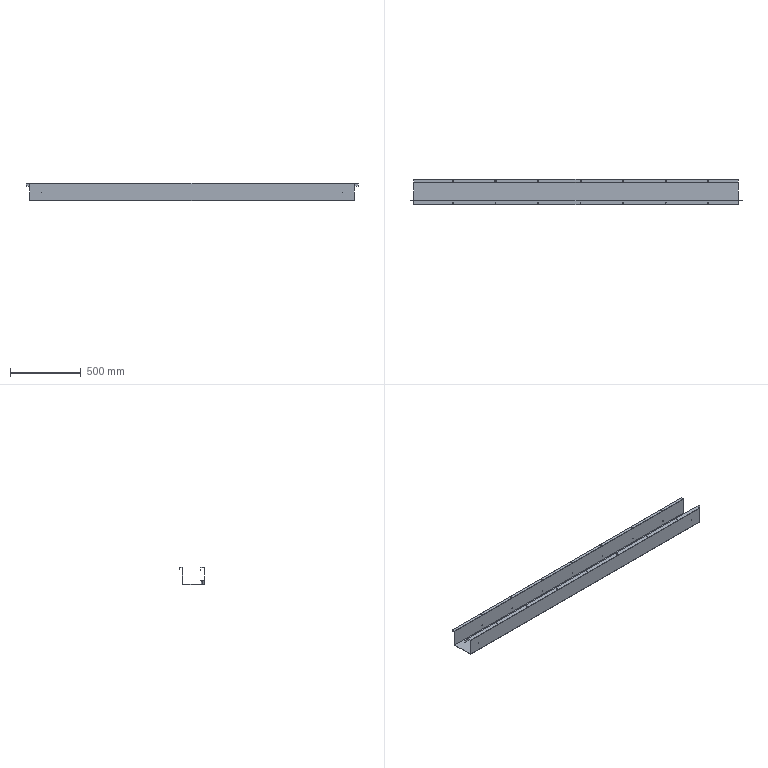Part | STEP file | SX-004-03 | 1 solid | 178 faces | box 2341 x 182.5 x 122 mm | volume 2234839 mm3 | cylinder 96 | plane 70 | cone 12 | commonest cylinder face diameters 5.4 x28 8 x14 8.5 x12 12.5 x12 20 x12 0.4 x6